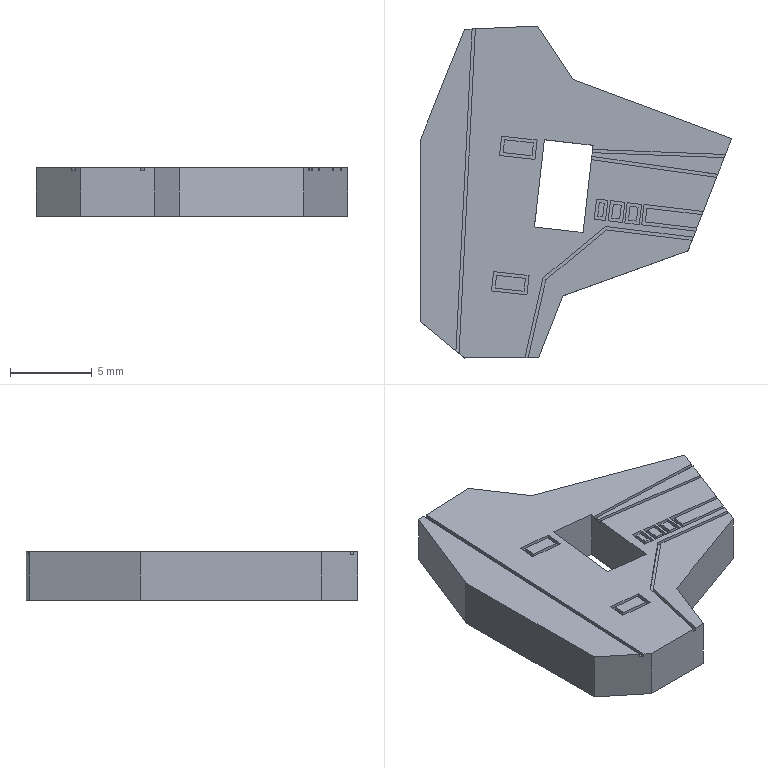Part | SolidWorks | features BaseBody 1 | 1 solid | 93 faces | box 19.081 x 20.339 x 3 mm | volume 705.753 mm3 | plane 84 | spline 9